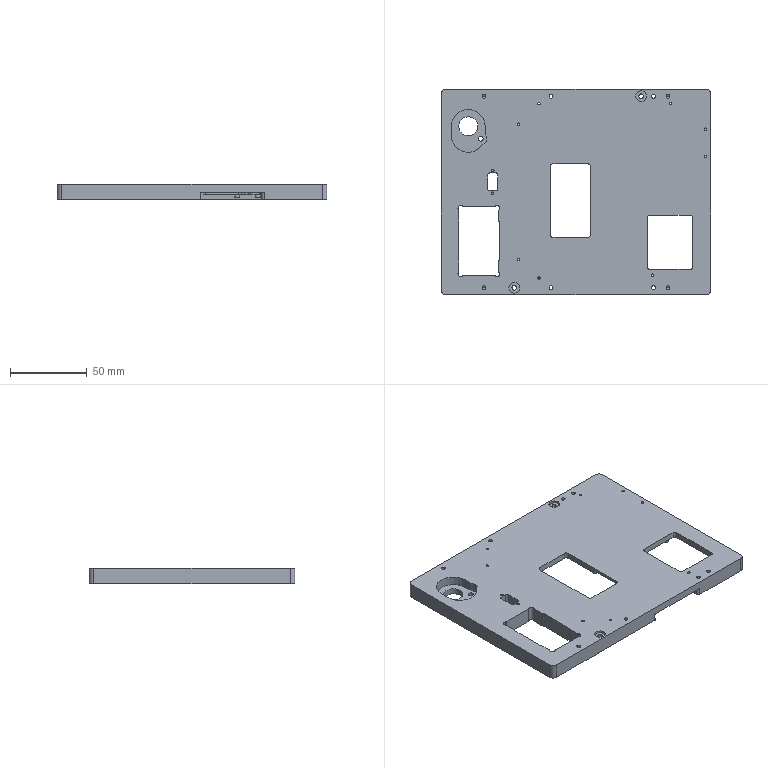NC program | NX | posted with a generic post | part box 176 x 134 x 10 mm
Lines 4859 to 5740 of 17594:
(CAVITY_MILL_COPY_COPY , TOOL : D4)
N9698 T17 M6
N9700 G54
N9702 G17 G0 G90 X-72.907 Y56.351 S9500 M3
N9704 G43 Z30. H17
N9706 Z-0.2
N9708 G94 G1 X-73.08 Y56.651 F1000.
N9710 G3 X-73.946 Y57.151 R1.
N9712 G1 X-75.237 F1400.
N9714 Y56.424
N9716 G2 X-75.278 Y55.89 R3.5
N9718 G3 X-74.916 Y54.958 R1.
N9720 G1 X-74.746 Y54.822
N9722 G0 X-72.907 Y56.351 Z-0.525
N9724 G1 X-73.08 Y56.651 F1000.
N9726 G3 X-73.946 Y57.151 R1.
N9728 G1 X-75.237 F1400.
N9730 Y56.424
N9732 G2 X-75.278 Y55.89 R3.5
N9734 G3 X-74.916 Y54.958 R1.
N9736 G1 X-74.746 Y54.822
N9738 G0 X-72.907 Y56.351 Z-0.85
N9740 G1 X-73.08 Y56.651 F1000.
N9742 G3 X-73.946 Y57.151 R1.
N9744 G1 X-75.237 F1400.
N9746 Y56.424
N9748 G2 X-75.278 Y55.89 R3.5
N9750 G3 X-74.916 Y54.958 R1.
N9752 G1 X-74.746 Y54.822
N9754 G0 X-72.907 Y56.351 Z-1.175
N9756 G1 X-73.08 Y56.651 F1000.
N9758 G3 X-73.946 Y57.151 R1.
N9760 G1 X-75.237 F1400.
N9762 Y56.424
N9764 G2 X-75.278 Y55.89 R3.5
N9766 G3 X-74.916 Y54.958 R1.
N9768 G1 X-74.746 Y54.822
N9770 G0 X-72.907 Y56.351 Z-1.5
N9772 G1 X-73.08 Y56.651 F1000.
N9774 G3 X-73.946 Y57.151 R1.
N9776 G1 X-75.237 F1400.
N9778 Y56.424
N9780 G2 X-75.278 Y55.89 R3.5
N9782 G3 X-74.916 Y54.958 R1.
N9784 G1 X-74.746 Y54.822
N9786 G0 X-72.907 Y56.351 Z-1.9
N9788 G1 X-73.08 Y56.651 F1000.
N9790 G3 X-73.946 Y57.151 R1.
N9792 G1 X-75.237 F1400.
N9794 Y56.424
N9796 G2 X-75.278 Y55.89 R3.5
N9798 G3 X-74.916 Y54.958 R1.
N9800 G1 X-74.746 Y54.822
N9802 G0 X-72.907 Y56.351 Z-2.3
N9804 G1 X-73.08 Y56.651 F1000.
N9806 G3 X-73.946 Y57.151 R1.
N9808 G1 X-75.237 F1400.
N9810 Y56.424
N9812 G2 X-75.278 Y55.89 R3.5
N9814 G3 X-74.916 Y54.958 R1.
N9816 G1 X-74.746 Y54.822
N9818 G0 X-72.907 Y56.351 Z-2.7
N9820 G1 X-73.08 Y56.651 F1000.
N9822 G3 X-73.946 Y57.151 R1.
N9824 G1 X-75.237 F1400.
N9826 Y56.424
N9828 G2 X-75.278 Y55.89 R3.5
N9830 G3 X-74.916 Y54.958 R1.
N9832 G1 X-74.746 Y54.822
N9834 G0 X-72.907 Y56.351 Z-3.1
N9836 G1 X-73.08 Y56.651 F1000.
N9838 G3 X-73.946 Y57.151 R1.
N9840 G1 X-75.237 F1400.
N9842 Y56.424
N9844 G2 X-75.278 Y55.89 R3.5
N9846 G3 X-74.916 Y54.958 R1.
N9848 G1 X-74.746 Y54.822
N9850 G0 Z30.
N9852 X-76.604 Y50.586
N9854 Z-3.35
N9856 G1 X-76.304 Y50.759 F1000.
N9858 G3 X-75.804 Y51.625 R1.
N9860 G1 Y52.924 F1400.
N9862 X-77.103
N9864 G3 X-77.969 Y52.424 R1.
N9866 G1 X-78.142 Y52.124
N9868 G0 X-76.604 Y50.586 Z-3.6
N9870 G1 X-76.304 Y50.759 F1000.
N9872 G3 X-75.804 Y51.625 R1.
N9874 G1 Y52.924 F1400.
N9876 X-77.103
N9878 G3 X-77.969 Y52.424 R1.
N9880 G1 X-78.142 Y52.124
N9882 G0 X-76.604 Y50.586 Z-3.933
N9884 G1 X-76.304 Y50.759 F1000.
N9886 G3 X-75.804 Y51.625 R1.
N9888 G1 Y52.924 F1400.
N9890 X-77.103
N9892 G3 X-77.969 Y52.424 R1.
N9894 G1 X-78.142 Y52.124
N9896 G0 X-76.604 Y50.586 Z-4.267
N9898 G1 X-76.304 Y50.759 F1000.
N9900 G3 X-75.804 Y51.625 R1.
N9902 G1 Y52.924 F1400.
N9904 X-77.103
N9906 G3 X-77.969 Y52.424 R1.
N9908 G1 X-78.142 Y52.124
N9910 G0 X-76.604 Y50.586 Z-4.6
N9912 G1 X-76.304 Y50.759 F1000.
N9914 G3 X-75.804 Y51.625 R1.
N9916 G1 Y52.924 F1400.
N9918 X-77.103
N9920 G3 X-77.969 Y52.424 R1.
N9922 G1 X-78.142 Y52.124
N9924 G0 X-76.604 Y50.586 Z-4.8
N9926 G1 X-76.304 Y50.759 F1000.
N9928 G3 X-75.804 Y51.625 R1.
N9930 G1 Y52.924 F1400.
N9932 X-77.103
N9934 G3 X-77.969 Y52.424 R1.
N9936 G1 X-78.142 Y52.124
N9938 G0 X-76.604 Y50.586 Z-5.
N9940 G1 X-76.304 Y50.759 F1000.
N9942 G3 X-75.804 Y51.625 R1.
N9944 G1 Y52.924 F1400.
N9946 X-77.103
N9948 G3 X-77.969 Y52.424 R1.
N9950 G1 X-78.142 Y52.124
N9952 G0 Z30.
N9954 X-67.1 Y49.336
N9956 Z-3.35
N9958 G1 X-67.273 Y49.636 F1000.
N9960 G3 X-68.139 Y50.136 R1.
N9962 G1 X-69.438 F1400.
N9964 Y48.837
N9966 G3 X-68.938 Y47.971 R1.
N9968 G1 X-68.638 Y47.798
N9970 G0 X-67.1 Y49.336 Z-3.6
N9972 G1 X-67.273 Y49.636 F1000.
N9974 G3 X-68.139 Y50.136 R1.
N9976 G1 X-69.438 F1400.
N9978 Y48.837
N9980 G3 X-68.938 Y47.971 R1.
N9982 G1 X-68.638 Y47.798
N9984 G0 X-67.1 Y49.336 Z-3.933
N9986 G1 X-67.273 Y49.636 F1000.
N9988 G3 X-68.139 Y50.136 R1.
N9990 G1 X-69.438 F1400.
N9992 Y48.837
N9994 G3 X-68.938 Y47.971 R1.
N9996 G1 X-68.638 Y47.798
N9998 G0 X-67.1 Y49.336 Z-4.267
N10000 G1 X-67.273 Y49.636 F1000.
N10002 G3 X-68.139 Y50.136 R1.
N10004 G1 X-69.438 F1400.
N10006 Y48.837
N10008 G3 X-68.938 Y47.971 R1.
N10010 G1 X-68.638 Y47.798
N10012 G0 X-67.1 Y49.336 Z-4.6
N10014 G1 X-67.273 Y49.636 F1000.
N10016 G3 X-68.139 Y50.136 R1.
N10018 G1 X-69.438 F1400.
N10020 Y48.837
N10022 G3 X-68.938 Y47.971 R1.
N10024 G1 X-68.638 Y47.798
N10026 G0 X-67.1 Y49.336 Z-4.8
N10028 G1 X-67.273 Y49.636 F1000.
N10030 G3 X-68.139 Y50.136 R1.
N10032 G1 X-69.438 F1400.
N10034 Y48.837
N10036 G3 X-68.938 Y47.971 R1.
N10038 G1 X-68.638 Y47.798
N10040 G0 Z30.
N10042 X-67.1 Y49.336
N10044 Z-5.1
N10046 G1 X-67.273 Y49.636 F1000.
N10048 G3 X-68.139 Y50.136 R1.
N10050 G1 X-69.438 F1400.
N10052 Y48.837
N10054 G3 X-68.938 Y47.971 R1.
N10056 G1 X-68.638 Y47.798
N10058 G0 X-67.1 Y49.336 Z-5.433
N10060 G1 X-67.273 Y49.636 F1000.
N10062 G3 X-68.139 Y50.136 R1.
N10064 G1 X-69.438 F1400.
N10066 Y48.837
N10068 G3 X-68.938 Y47.971 R1.
N10070 G1 X-68.638 Y47.798
N10072 G0 X-67.1 Y49.336 Z-5.767
N10074 G1 X-67.273 Y49.636 F1000.
N10076 G3 X-68.139 Y50.136 R1.
N10078 G1 X-69.438 F1400.
N10080 Y48.837
N10082 G3 X-68.938 Y47.971 R1.
N10084 G1 X-68.638 Y47.798
N10086 G0 X-67.1 Y49.336 Z-6.1
N10088 G1 X-67.273 Y49.636 F1000.
N10090 G3 X-68.139 Y50.136 R1.
N10092 G1 X-69.438 F1400.
N10094 Y48.837
N10096 G3 X-68.938 Y47.971 R1.
N10098 G1 X-68.638 Y47.798
N10100 G0 Z30.
N10102 Y41.785
N10104 Z-3.35
N10106 G1 X-68.938 Y41.612 F1000.
N10108 G3 X-69.438 Y40.746 R1.
N10110 G1 Y39.447 F1400.
N10112 X-68.139
N10114 G3 X-67.273 Y39.947 R1.
N10116 G1 X-67.1 Y40.247
N10118 G0 X-68.638 Y41.785 Z-3.6
N10120 G1 X-68.938 Y41.612 F1000.
N10122 G3 X-69.438 Y40.746 R1.
N10124 G1 Y39.447 F1400.
N10126 X-68.139
N10128 G3 X-67.273 Y39.947 R1.
N10130 G1 X-67.1 Y40.247
N10132 G0 X-68.638 Y41.785 Z-3.933
N10134 G1 X-68.938 Y41.612 F1000.
N10136 G3 X-69.438 Y40.746 R1.
N10138 G1 Y39.447 F1400.
N10140 X-68.139
N10142 G3 X-67.273 Y39.947 R1.
N10144 G1 X-67.1 Y40.247
N10146 G0 X-68.638 Y41.785 Z-4.267
N10148 G1 X-68.938 Y41.612 F1000.
N10150 G3 X-69.438 Y40.746 R1.
N10152 G1 Y39.447 F1400.
N10154 X-68.139
N10156 G3 X-67.273 Y39.947 R1.
N10158 G1 X-67.1 Y40.247
N10160 G0 X-68.638 Y41.785 Z-4.6
N10162 G1 X-68.938 Y41.612 F1000.
N10164 G3 X-69.438 Y40.746 R1.
N10166 G1 Y39.447 F1400.
N10168 X-68.139
N10170 G3 X-67.273 Y39.947 R1.
N10172 G1 X-67.1 Y40.247
N10174 G0 X-68.638 Y41.785 Z-4.8
N10176 G1 X-68.938 Y41.612 F1000.
N10178 G3 X-69.438 Y40.746 R1.
N10180 G1 Y39.447 F1400.
N10182 X-68.139
N10184 G3 X-67.273 Y39.947 R1.
N10186 G1 X-67.1 Y40.247
N10188 G0 Z30.
N10190 X-68.638 Y41.785
N10192 Z-5.1
N10194 G1 X-68.938 Y41.612 F1000.
N10196 G3 X-69.438 Y40.746 R1.
N10198 G1 Y39.447 F1400.
N10200 X-68.139
N10202 G3 X-67.273 Y39.947 R1.
N10204 G1 X-67.1 Y40.247
N10206 G0 X-68.638 Y41.785 Z-5.433
N10208 G1 X-68.938 Y41.612 F1000.
N10210 G3 X-69.438 Y40.746 R1.
N10212 G1 Y39.447 F1400.
N10214 X-68.139
N10216 G3 X-67.273 Y39.947 R1.
N10218 G1 X-67.1 Y40.247
N10220 G0 X-68.638 Y41.785 Z-5.767
N10222 G1 X-68.938 Y41.612 F1000.
N10224 G3 X-69.438 Y40.746 R1.
N10226 G1 Y39.447 F1400.
N10228 X-68.139
N10230 G3 X-67.273 Y39.947 R1.
N10232 G1 X-67.1 Y40.247
N10234 G0 X-68.638 Y41.785 Z-6.1
N10236 G1 X-68.938 Y41.612 F1000.
N10238 G3 X-69.438 Y40.746 R1.
N10240 G1 Y39.447 F1400.
N10242 X-68.139
N10244 G3 X-67.273 Y39.947 R1.
N10246 G1 X-67.1 Y40.247
N10248 G0 Z30.
N10250 X-72.898 Y25.976
N10252 Z-5.1
N10254 G1 X-73.072 Y26.276 F1000.
N10256 G3 X-73.938 Y26.776 R1.
N10258 G1 X-75.237 F1400.
N10260 Y25.477
N10262 G3 X-74.737 Y24.611 R1.
N10264 G1 X-74.437 Y24.437
N10266 G0 X-72.898 Y25.976 Z-5.433
N10268 G1 X-73.072 Y26.276 F1000.
N10270 G3 X-73.938 Y26.776 R1.
N10272 G1 X-75.237 F1400.
N10274 Y25.477
N10276 G3 X-74.737 Y24.611 R1.
N10278 G1 X-74.437 Y24.437
N10280 G0 X-72.898 Y25.976 Z-5.767
N10282 G1 X-73.072 Y26.276 F1000.
N10284 G3 X-73.938 Y26.776 R1.
N10286 G1 X-75.237 F1400.
N10288 Y25.477
N10290 G3 X-74.737 Y24.611 R1.
N10292 G1 X-74.437 Y24.437
N10294 G0 X-72.898 Y25.976 Z-6.1
N10296 G1 X-73.072 Y26.276 F1000.
N10298 G3 X-73.938 Y26.776 R1.
N10300 G1 X-75.237 F1400.
N10302 Y25.477
N10304 G3 X-74.737 Y24.611 R1.
N10306 G1 X-74.437 Y24.437
N10308 G0 Z30.
N10310 X-61.137 Y18.058
N10312 Z-6.5
N10314 G1 X-61.437 Y17.885 F1000.
N10316 G3 X-61.937 Y17.019 R1.
N10318 G1 Y15.72 F1400.
N10320 X-60.638
N10322 G3 X-59.772 Y16.22 R1.
N10324 G1 X-59.599 Y16.52
N10326 G0 X-61.137 Y18.058 Z-6.9
N10328 G1 X-61.437 Y17.885 F1000.
N10330 G3 X-61.937 Y17.019 R1.
N10332 G1 Y15.72 F1400.
N10334 X-60.638
N10336 G3 X-59.772 Y16.22 R1.
N10338 G1 X-59.599 Y16.52
N10340 G0 X-61.137 Y18.058 Z-7.3
N10342 G1 X-61.437 Y17.885 F1000.
N10344 G3 X-61.937 Y17.019 R1.
N10346 G1 Y15.72 F1400.
N10348 X-60.638
N10350 G3 X-59.772 Y16.22 R1.
N10352 G1 X-59.599 Y16.52
N10354 G0 X-61.137 Y18.058 Z-7.7
N10356 G1 X-61.437 Y17.885 F1000.
N10358 G3 X-61.937 Y17.019 R1.
N10360 G1 Y15.72 F1400.
N10362 X-60.638
N10364 G3 X-59.772 Y16.22 R1.
N10366 G1 X-59.599 Y16.52
N10368 G0 X-61.137 Y18.058 Z-8.1
N10370 G1 X-61.437 Y17.885 F1000.
N10372 G3 X-61.937 Y17.019 R1.
N10374 G1 Y15.72 F1400.
N10376 X-60.638
N10378 G3 X-59.772 Y16.22 R1.
N10380 G1 X-59.599 Y16.52
N10382 G0 Z30.
N10384 X-59.989 Y28.441
N10386 Z-3.35
N10388 G1 X-60.162 Y28.741 F1000.
N10390 G3 X-61.028 Y29.241 R1.
N10392 G1 X-61.997 F1400.
N10394 G2 X-62.378 Y28.412 R3.5
N10396 G3 X-62.416 Y27.413 R1.
N10398 G1 X-62.315 Y27.221
N10400 G0 X-59.989 Y28.441 Z-3.6
N10402 G1 X-60.162 Y28.741 F1000.
N10404 G3 X-61.028 Y29.241 R1.
N10406 G1 X-61.997 F1400.
N10408 G2 X-62.378 Y28.412 R3.5
N10410 G3 X-62.416 Y27.413 R1.
N10412 G1 X-62.315 Y27.221
N10414 G0 X-59.989 Y28.441 Z-3.933
N10416 G1 X-60.162 Y28.741 F1000.
N10418 G3 X-61.028 Y29.241 R1.
N10420 G1 X-61.997 F1400.
N10422 G2 X-62.378 Y28.412 R3.5
N10424 G3 X-62.416 Y27.413 R1.
N10426 G1 X-62.315 Y27.221
N10428 G0 X-59.989 Y28.441 Z-4.267
N10430 G1 X-60.162 Y28.741 F1000.
N10432 G3 X-61.028 Y29.241 R1.
N10434 G1 X-61.997 F1400.
N10436 G2 X-62.378 Y28.412 R3.5
N10438 G3 X-62.416 Y27.413 R1.
N10440 G1 X-62.315 Y27.221
N10442 G0 X-59.989 Y28.441 Z-4.6
N10444 G1 X-60.162 Y28.741 F1000.
N10446 G3 X-61.028 Y29.241 R1.
N10448 G1 X-61.997 F1400.
N10450 G2 X-62.378 Y28.412 R3.5
N10452 G3 X-62.416 Y27.413 R1.
N10454 G1 X-62.315 Y27.221
N10456 G0 X-59.989 Y28.441 Z-4.8
N10458 G1 X-60.162 Y28.741 F1000.
N10460 G3 X-61.028 Y29.241 R1.
N10462 G1 X-61.997 F1400.
N10464 G2 X-62.378 Y28.412 R3.5
N10466 G3 X-62.416 Y27.413 R1.
N10468 G1 X-62.315 Y27.221
N10470 G0 Z30.
N10472 X-59.989 Y28.441
N10474 Z-5.1
N10476 G1 X-60.162 Y28.741 F1000.
N10478 G3 X-61.028 Y29.241 R1.
N10480 G1 X-61.997 F1400.
N10482 G2 X-62.378 Y28.412 R3.5
N10484 G3 X-62.416 Y27.413 R1.
N10486 G1 X-62.315 Y27.221
N10488 G0 X-59.989 Y28.441 Z-5.433
N10490 G1 X-60.162 Y28.741 F1000.
N10492 G3 X-61.028 Y29.241 R1.
N10494 G1 X-61.997 F1400.
N10496 G2 X-62.378 Y28.412 R3.5
N10498 G3 X-62.416 Y27.413 R1.
N10500 G1 X-62.315 Y27.221
N10502 G0 X-59.989 Y28.441 Z-5.767
N10504 G1 X-60.162 Y28.741 F1000.
N10506 G3 X-61.028 Y29.241 R1.
N10508 G1 X-61.997 F1400.
N10510 G2 X-62.378 Y28.412 R3.5
N10512 G3 X-62.416 Y27.413 R1.
N10514 G1 X-62.315 Y27.221
N10516 G0 X-59.989 Y28.441 Z-6.1
N10518 G1 X-60.162 Y28.741 F1000.
N10520 G3 X-61.028 Y29.241 R1.
N10522 G1 X-61.997 F1400.
N10524 G2 X-62.378 Y28.412 R3.5
N10526 G3 X-62.416 Y27.413 R1.
N10528 G1 X-62.315 Y27.221
N10530 G0 Z30.
N10532 X-59.599 Y28.441
N10534 Z-6.5
N10536 G1 X-59.772 Y28.741 F1000.
N10538 G3 X-60.638 Y29.241 R1.
N10540 G1 X-61.937 F1400.
N10542 Y27.942
N10544 G3 X-61.437 Y27.076 R1.
N10546 G1 X-61.137 Y26.903
N10548 G0 X-59.599 Y28.441 Z-6.9
N10550 G1 X-59.772 Y28.741 F1000.
N10552 G3 X-60.638 Y29.241 R1.
N10554 G1 X-61.937 F1400.
N10556 Y27.942
N10558 G3 X-61.437 Y27.076 R1.
N10560 G1 X-61.137 Y26.903
N10562 G0 X-59.599 Y28.441 Z-7.3
N10564 G1 X-59.772 Y28.741 F1000.
N10566 G3 X-60.638 Y29.241 R1.
N10568 G1 X-61.937 F1400.
N10570 Y27.942
N10572 G3 X-61.437 Y27.076 R1.
N10574 G1 X-61.137 Y26.903
N10576 G0 X-59.599 Y28.441 Z-7.7
N10578 G1 X-59.772 Y28.741 F1000.
N10580 G3 X-60.638 Y29.241 R1.
N10582 G1 X-61.937 F1400.
N10584 Y27.942
N10586 G3 X-61.437 Y27.076 R1.
N10588 G1 X-61.137 Y26.903
N10590 G0 X-59.599 Y28.441 Z-8.1
N10592 G1 X-59.772 Y28.741 F1000.
N10594 G3 X-60.638 Y29.241 R1.
N10596 G1 X-61.937 F1400.
N10598 Y27.942
N10600 G3 X-61.437 Y27.076 R1.
N10602 G1 X-61.137 Y26.903
N10604 G0 Z30.
N10606 X-66.52 Y40.247
N10608 Z-3.35
N10610 G1 X-66.347 Y39.947 F1000.
N10612 G3 X-65.481 Y39.447 R1.
N10614 G1 X-64.182 F1400.
N10616 Y40.746
N10618 G3 X-64.682 Y41.612 R1.
N10620 G1 X-64.982 Y41.785
N10622 G0 X-66.52 Y40.247 Z-3.6
N10624 G1 X-66.347 Y39.947 F1000.
N10626 G3 X-65.481 Y39.447 R1.
N10628 G1 X-64.182 F1400.
N10630 Y40.746
N10632 G3 X-64.682 Y41.612 R1.
N10634 G1 X-64.982 Y41.785
N10636 G0 X-66.52 Y40.247 Z-3.933
N10638 G1 X-66.347 Y39.947 F1000.
N10640 G3 X-65.481 Y39.447 R1.
N10642 G1 X-64.182 F1400.
N10644 Y40.746
N10646 G3 X-64.682 Y41.612 R1.
N10648 G1 X-64.982 Y41.785
N10650 G0 X-66.52 Y40.247 Z-4.267
N10652 G1 X-66.347 Y39.947 F1000.
N10654 G3 X-65.481 Y39.447 R1.
N10656 G1 X-64.182 F1400.
N10658 Y40.746
N10660 G3 X-64.682 Y41.612 R1.
N10662 G1 X-64.982 Y41.785
N10664 G0 X-66.52 Y40.247 Z-4.6
N10666 G1 X-66.347 Y39.947 F1000.
N10668 G3 X-65.481 Y39.447 R1.
N10670 G1 X-64.182 F1400.
N10672 Y40.746
N10674 G3 X-64.682 Y41.612 R1.
N10676 G1 X-64.982 Y41.785
N10678 G0 X-66.52 Y40.247 Z-4.8
N10680 G1 X-66.347 Y39.947 F1000.
N10682 G3 X-65.481 Y39.447 R1.
N10684 G1 X-64.182 F1400.
N10686 Y40.746
N10688 G3 X-64.682 Y41.612 R1.
N10690 G1 X-64.982 Y41.785
N10692 G0 Z30.
N10694 X-66.52 Y40.247
N10696 Z-5.1
N10698 G1 X-66.347 Y39.947 F1000.
N10700 G3 X-65.481 Y39.447 R1.
N10702 G1 X-64.182 F1400.
N10704 Y40.746
N10706 G3 X-64.682 Y41.612 R1.
N10708 G1 X-64.982 Y41.785
N10710 G0 X-66.52 Y40.247 Z-5.433
N10712 G1 X-66.347 Y39.947 F1000.
N10714 G3 X-65.481 Y39.447 R1.
N10716 G1 X-64.182 F1400.
N10718 Y40.746
N10720 G3 X-64.682 Y41.612 R1.
N10722 G1 X-64.982 Y41.785
N10724 G0 X-66.52 Y40.247 Z-5.767
N10726 G1 X-66.347 Y39.947 F1000.
N10728 G3 X-65.481 Y39.447 R1.
N10730 G1 X-64.182 F1400.
N10732 Y40.746
N10734 G3 X-64.682 Y41.612 R1.
N10736 G1 X-64.982 Y41.785
N10738 G0 X-66.52 Y40.247 Z-6.1
N10740 G1 X-66.347 Y39.947 F1000.
N10742 G3 X-65.481 Y39.447 R1.
N10744 G1 X-64.182 F1400.
N10746 Y40.746
N10748 G3 X-64.682 Y41.612 R1.
N10750 G1 X-64.982 Y41.785
N10752 G0 Z30.
N10754 Y47.798
N10756 Z-3.35
N10758 G1 X-64.682 Y47.971 F1000.
N10760 G3 X-64.182 Y48.837 R1.
N10762 G1 Y50.136 F1400.
N10764 X-65.481
N10766 G3 X-66.347 Y49.636 R1.
N10768 G1 X-66.52 Y49.336
N10770 G0 X-64.982 Y47.798 Z-3.6
N10772 G1 X-64.682 Y47.971 F1000.
N10774 G3 X-64.182 Y48.837 R1.
N10776 G1 Y50.136 F1400.
N10778 X-65.481
N10780 G3 X-66.347 Y49.636 R1.
N10782 G1 X-66.52 Y49.336
N10784 G0 X-64.982 Y47.798 Z-3.933
N10786 G1 X-64.682 Y47.971 F1000.
N10788 G3 X-64.182 Y48.837 R1.
N10790 G1 Y50.136 F1400.
N10792 X-65.481
N10794 G3 X-66.347 Y49.636 R1.
N10796 G1 X-66.52 Y49.336
N10798 G0 X-64.982 Y47.798 Z-4.267
N10800 G1 X-64.682 Y47.971 F1000.
N10802 G3 X-64.182 Y48.837 R1.
N10804 G1 Y50.136 F1400.
N10806 X-65.481
N10808 G3 X-66.347 Y49.636 R1.
N10810 G1 X-66.52 Y49.336
N10812 G0 X-64.982 Y47.798 Z-4.6
N10814 G1 X-64.682 Y47.971 F1000.
N10816 G3 X-64.182 Y48.837 R1.
N10818 G1 Y50.136 F1400.
N10820 X-65.481
N10822 G3 X-66.347 Y49.636 R1.
N10824 G1 X-66.52 Y49.336
N10826 G0 X-64.982 Y47.798 Z-4.8
N10828 G1 X-64.682 Y47.971 F1000.
N10830 G3 X-64.182 Y48.837 R1.
N10832 G1 Y50.136 F1400.
N10834 X-65.481
N10836 G3 X-66.347 Y49.636 R1.
N10838 G1 X-66.52 Y49.336
N10840 G0 Z30.
N10842 X-64.982 Y47.798
N10844 Z-5.1
N10846 G1 X-64.682 Y47.971 F1000.
N10848 G3 X-64.182 Y48.837 R1.
N10850 G1 Y50.136 F1400.
N10852 X-65.481
N10854 G3 X-66.347 Y49.636 R1.
N10856 G1 X-66.52 Y49.336
N10858 G0 X-64.982 Y47.798 Z-5.433
N10860 G1 X-64.682 Y47.971 F1000.
N10862 G3 X-64.182 Y48.837 R1.
N10864 G1 Y50.136 F1400.
N10866 X-65.481
N10868 G3 X-66.347 Y49.636 R1.
N10870 G1 X-66.52 Y49.336
N10872 G0 X-64.982 Y47.798 Z-5.767
N10874 G1 X-64.682 Y47.971 F1000.
N10876 G3 X-64.182 Y48.837 R1.
N10878 G1 Y50.136 F1400.
N10880 X-65.481
N10882 G3 X-66.347 Y49.636 R1.
N10884 G1 X-66.52 Y49.336
N10886 G0 X-64.982 Y47.798 Z-6.1
N10888 G1 X-64.682 Y47.971 F1000.
N10890 G3 X-64.182 Y48.837 R1.
N10892 G1 Y50.136 F1400.
N10894 X-65.481
N10896 G3 X-66.347 Y49.636 R1.
N10898 G1 X-66.52 Y49.336
N10900 G0 Z30.
N10902 X-60.387 Y56.351
N10904 Z-1.9
N10906 G1 X-60.474 Y56.568 F1000.
N10908 G3 X-61.26 Y57.186 R1.
N10910 G2 X-61.81 Y57.312 R3.5 F1400.
N10912 X-62.361 Y57.186 R3.5
N10914 G3 X-63.147 Y56.568 R1.
N10916 G1 X-63.234 Y56.351
N10918 G0 X-60.387 Z-2.3
N10920 G1 X-60.474 Y56.568 F1000.
N10922 G3 X-61.26 Y57.186 R1.
N10924 G2 X-61.81 Y57.312 R3.5 F1400.
N10926 X-62.361 Y57.186 R3.5
N10928 G3 X-63.147 Y56.568 R1.
N10930 G1 X-63.234 Y56.351
N10932 G0 X-60.387 Z-2.7
N10934 G1 X-60.474 Y56.568 F1000.
N10936 G3 X-61.26 Y57.186 R1.
N10938 G2 X-61.81 Y57.312 R3.5 F1400.
N10940 X-62.361 Y57.186 R3.5
N10942 G3 X-63.147 Y56.568 R1.
N10944 G1 X-63.234 Y56.351
N10946 G0 X-60.387 Z-3.1
N10948 G1 X-60.474 Y56.568 F1000.
N10950 G3 X-61.26 Y57.186 R1.
N10952 G2 X-61.81 Y57.312 R3.5 F1400.
N10954 X-62.361 Y57.186 R3.5
N10956 G3 X-63.147 Y56.568 R1.
N10958 G1 X-63.234 Y56.351
N10960 G0 Z30.
N10962 X-36.331 Y52.148
N10964 Z-3.35
N10966 G1 X-36.505 Y52.448 F1000.
N10968 G3 X-37.371 Y52.948 R1.
N10970 G1 X-38.67 F1400.
N10972 Y51.649
N10974 G3 X-38.17 Y50.783 R1.
N10976 G1 X-37.87 Y50.609
N10978 G0 X-36.331 Y52.148 Z-3.6
N10980 G1 X-36.505 Y52.448 F1000.
N10982 G3 X-37.371 Y52.948 R1.
N10984 G1 X-38.67 F1400.
N10986 Y51.649
N10988 G3 X-38.17 Y50.783 R1.
N10990 G1 X-37.87 Y50.609
N10992 G0 X-36.331 Y52.148 Z-3.933
N10994 G1 X-36.505 Y52.448 F1000.
N10996 G3 X-37.371 Y52.948 R1.
N10998 G1 X-38.67 F1400.
N11000 Y51.649
N11002 G3 X-38.17 Y50.783 R1.
N11004 G1 X-37.87 Y50.609
N11006 G0 X-36.331 Y52.148 Z-4.267
N11008 G1 X-36.505 Y52.448 F1000.
N11010 G3 X-37.371 Y52.948 R1.
N11012 G1 X-38.67 F1400.
N11014 Y51.649
N11016 G3 X-38.17 Y50.783 R1.
N11018 G1 X-37.87 Y50.609
N11020 G0 X-36.331 Y52.148 Z-4.6
N11022 G1 X-36.505 Y52.448 F1000.
N11024 G3 X-37.371 Y52.948 R1.
N11026 G1 X-38.67 F1400.
N11028 Y51.649
N11030 G3 X-38.17 Y50.783 R1.
N11032 G1 X-37.87 Y50.609
N11034 G0 X-36.331 Y52.148 Z-4.8
N11036 G1 X-36.505 Y52.448 F1000.
N11038 G3 X-37.371 Y52.948 R1.
N11040 G1 X-38.67 F1400.
N11042 Y51.649
N11044 G3 X-38.17 Y50.783 R1.
N11046 G1 X-37.87 Y50.609
N11048 G0 Z30.
N11050 X-36.331 Y52.148
N11052 Z-5.1
N11054 G1 X-36.505 Y52.448 F1000.
N11056 G3 X-37.371 Y52.948 R1.
N11058 G1 X-38.67 F1400.
N11060 Y51.649
N11062 G3 X-38.17 Y50.783 R1.
N11064 G1 X-37.87 Y50.609
N11066 G0 X-36.331 Y52.148 Z-5.433
N11068 G1 X-36.505 Y52.448 F1000.
N11070 G3 X-37.371 Y52.948 R1.
N11072 G1 X-38.67 F1400.
N11074 Y51.649
N11076 G3 X-38.17 Y50.783 R1.
N11078 G1 X-37.87 Y50.609
N11080 G0 X-36.331 Y52.148 Z-5.767
N11082 G1 X-36.505 Y52.448 F1000.
N11084 G3 X-37.371 Y52.948 R1.
N11086 G1 X-38.67 F1400.
N11088 Y51.649
N11090 G3 X-38.17 Y50.783 R1.
N11092 G1 X-37.87 Y50.609
N11094 G0 X-36.331 Y52.148 Z-6.1
N11096 G1 X-36.505 Y52.448 F1000.
N11098 G3 X-37.371 Y52.948 R1.
N11100 G1 X-38.67 F1400.
N11102 Y51.649
N11104 G3 X-38.17 Y50.783 R1.
N11106 G1 X-37.87 Y50.609
N11108 G0 X-36.331 Y52.148 Z-6.5
N11110 G1 X-36.505 Y52.448 F1000.
N11112 G3 X-37.371 Y52.948 R1.
N11114 G1 X-38.67 F1400.
N11116 Y51.649
N11118 G3 X-38.17 Y50.783 R1.
N11120 G1 X-37.87 Y50.609
N11122 G0 X-36.331 Y52.148 Z-6.9
N11124 G1 X-36.505 Y52.448 F1000.
N11126 G3 X-37.371 Y52.948 R1.
N11128 G1 X-38.67 F1400.
N11130 Y51.649
N11132 G3 X-38.17 Y50.783 R1.
N11134 G1 X-37.87 Y50.609
N11136 G0 X-36.331 Y52.148 Z-7.3
N11138 G1 X-36.505 Y52.448 F1000.
N11140 G3 X-37.371 Y52.948 R1.
N11142 G1 X-38.67 F1400.
N11144 Y51.649
N11146 G3 X-38.17 Y50.783 R1.
N11148 G1 X-37.87 Y50.609
N11150 G0 X-36.331 Y52.148 Z-7.7
N11152 G1 X-36.505 Y52.448 F1000.
N11154 G3 X-37.371 Y52.948 R1.
N11156 G1 X-38.67 F1400.
N11158 Y51.649
N11160 G3 X-38.17 Y50.783 R1.
N11162 G1 X-37.87 Y50.609
N11164 G0 X-36.331 Y52.148 Z-8.1
N11166 G1 X-36.505 Y52.448 F1000.
N11168 G3 X-37.371 Y52.948 R1.
N11170 G1 X-38.67 F1400.
N11172 Y51.649
N11174 G3 X-38.17 Y50.783 R1.
N11176 G1 X-37.87 Y50.609
N11178 G0 Z30.
N11180 X-8.117
N11182 Z-3.35
N11184 G1 X-7.817 Y50.783 F1000.
N11186 G3 X-7.317 Y51.649 R1.
N11188 G1 Y52.948 F1400.
N11190 X-8.616
N11192 G3 X-9.482 Y52.448 R1.
N11194 G1 X-9.655 Y52.148
N11196 G0 X-8.117 Y50.609 Z-3.6
N11198 G1 X-7.817 Y50.783 F1000.
N11200 G3 X-7.317 Y51.649 R1.
N11202 G1 Y52.948 F1400.
N11204 X-8.616
N11206 G3 X-9.482 Y52.448 R1.
N11208 G1 X-9.655 Y52.148
N11210 G0 X-8.117 Y50.609 Z-3.933
N11212 G1 X-7.817 Y50.783 F1000.
N11214 G3 X-7.317 Y51.649 R1.
N11216 G1 Y52.948 F1400.
N11218 X-8.616
N11220 G3 X-9.482 Y52.448 R1.
N11222 G1 X-9.655 Y52.148
N11224 G0 X-8.117 Y50.609 Z-4.267
N11226 G1 X-7.817 Y50.783 F1000.
N11228 G3 X-7.317 Y51.649 R1.
N11230 G1 Y52.948 F1400.
N11232 X-8.616
N11234 G3 X-9.482 Y52.448 R1.
N11236 G1 X-9.655 Y52.148
N11238 G0 X-8.117 Y50.609 Z-4.6
N11240 G1 X-7.817 Y50.783 F1000.
N11242 G3 X-7.317 Y51.649 R1.
N11244 G1 Y52.948 F1400.
N11246 X-8.616
N11248 G3 X-9.482 Y52.448 R1.
N11250 G1 X-9.655 Y52.148
N11252 G0 X-8.117 Y50.609 Z-4.8
N11254 G1 X-7.817 Y50.783 F1000.
N11256 G3 X-7.317 Y51.649 R1.
N11258 G1 Y52.948 F1400.
N11260 X-8.616
N11262 G3 X-9.482 Y52.448 R1.
N11264 G1 X-9.655 Y52.148
N11266 G0 Z30.
N11268 X-8.117 Y50.609
N11270 Z-5.1
N11272 G1 X-7.817 Y50.783 F1000.
N11274 G3 X-7.317 Y51.649 R1.
N11276 G1 Y52.948 F1400.
N11278 X-8.616
N11280 G3 X-9.482 Y52.448 R1.
N11282 G1 X-9.655 Y52.148
N11284 G0 X-8.117 Y50.609 Z-5.433
N11286 G1 X-7.817 Y50.783 F1000.
N11288 G3 X-7.317 Y51.649 R1.
N11290 G1 Y52.948 F1400.
N11292 X-8.616
N11294 G3 X-9.482 Y52.448 R1.
N11296 G1 X-9.655 Y52.148
N11298 G0 X-8.117 Y50.609 Z-5.767
N11300 G1 X-7.817 Y50.783 F1000.
N11302 G3 X-7.317 Y51.649 R1.
N11304 G1 Y52.948 F1400.
N11306 X-8.616
N11308 G3 X-9.482 Y52.448 R1.
N11310 G1 X-9.655 Y52.148
N11312 G0 X-8.117 Y50.609 Z-6.1
N11314 G1 X-7.817 Y50.783 F1000.
N11316 G3 X-7.317 Y51.649 R1.
N11318 G1 Y52.948 F1400.
N11320 X-8.616
N11322 G3 X-9.482 Y52.448 R1.
N11324 G1 X-9.655 Y52.148
N11326 G0 X-8.117 Y50.609 Z-6.5
N11328 G1 X-7.817 Y50.783 F1000.
N11330 G3 X-7.317 Y51.649 R1.
N11332 G1 Y52.948 F1400.
N11334 X-8.616
N11336 G3 X-9.482 Y52.448 R1.
N11338 G1 X-9.655 Y52.148
N11340 G0 X-8.117 Y50.609 Z-6.9
N11342 G1 X-7.817 Y50.783 F1000.
N11344 G3 X-7.317 Y51.649 R1.
N11346 G1 Y52.948 F1400.
N11348 X-8.616
N11350 G3 X-9.482 Y52.448 R1.
N11352 G1 X-9.655 Y52.148
N11354 G0 X-8.117 Y50.609 Z-7.3
N11356 G1 X-7.817 Y50.783 F1000.
N11358 G3 X-7.317 Y51.649 R1.
N11360 G1 Y52.948 F1400.
N11362 X-8.616
N11364 G3 X-9.482 Y52.448 R1.
N11366 G1 X-9.655 Y52.148
N11368 G0 X-8.117 Y50.609 Z-7.7
N11370 G1 X-7.817 Y50.783 F1000.
N11372 G3 X-7.317 Y51.649 R1.
N11374 G1 Y52.948 F1400.
N11376 X-8.616
N11378 G3 X-9.482 Y52.448 R1.
N11380 G1 X-9.655 Y52.148
N11382 G0 X-8.117 Y50.609 Z-8.1
N11384 G1 X-7.817 Y50.783 F1000.
N11386 G3 X-7.317 Y51.649 R1.
N11388 G1 Y52.948 F1400.
N11390 X-8.616
N11392 G3 X-9.482 Y52.448 R1.
N11394 G1 X-9.655 Y52.148
N11396 G0 Z30.
N11398 X25.622 Y56.351
N11400 Z-1.9
N11402 G1 X25.55 Y56.559 F1000.
N11404 G3 X24.796 Y57.215 R1.
N11406 G2 X24.201 Y57.387 R3.5 F1400.
N11408 X23.606 Y57.215 R3.5
N11410 G3 X22.852 Y56.559 R1.
N11412 G1 X22.78 Y56.351
N11414 G0 X25.622 Z-2.3
N11416 G1 X25.55 Y56.559 F1000.
N11418 G3 X24.796 Y57.215 R1.
N11420 G2 X24.201 Y57.387 R3.5 F1400.
N11422 X23.606 Y57.215 R3.5
N11424 G3 X22.852 Y56.559 R1.
N11426 G1 X22.78 Y56.351
N11428 G0 X25.622 Z-2.7
N11430 G1 X25.55 Y56.559 F1000.
N11432 G3 X24.796 Y57.215 R1.
N11434 G2 X24.201 Y57.387 R3.5 F1400.
N11436 X23.606 Y57.215 R3.5
N11438 G3 X22.852 Y56.559 R1.
N11440 G1 X22.78 Y56.351
N11442 G0 X25.622 Z-3.1
N11444 G1 X25.55 Y56.559 F1000.
N11446 G3 X24.796 Y57.215 R1.
N11448 G2 X24.201 Y57.387 R3.5 F1400.
N11450 X23.606 Y57.215 R3.5
N11452 G3 X22.852 Y56.559 R1.
N11454 G1 X22.78 Y56.351